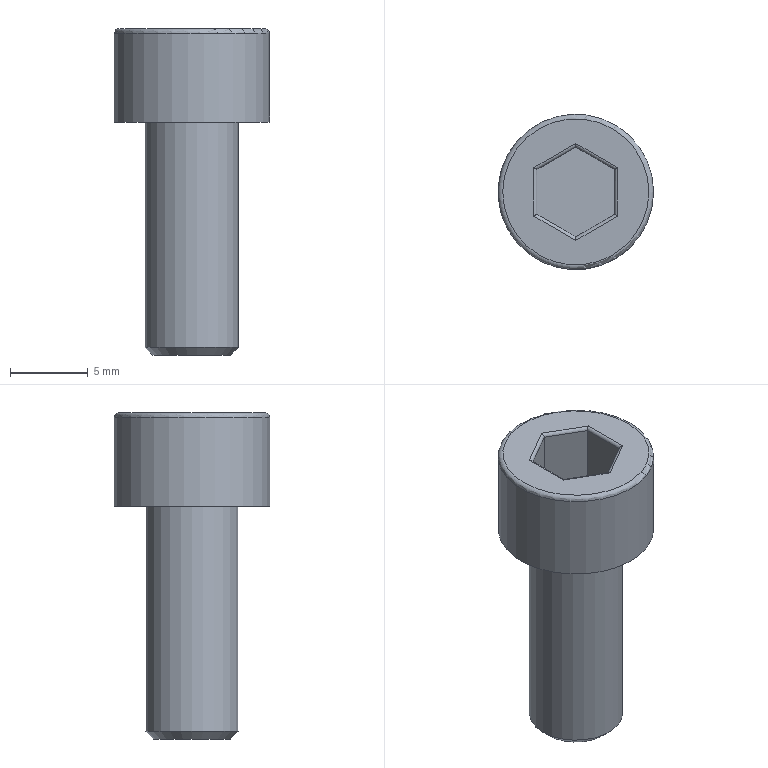Part | STEP file | 200 mesh_id126_x | 1 solid | 20 faces | box 10 x 10 x 21 mm | volume 805.776 mm3 | plane 10 | cylinder 8 | torus 1 | cone 1 | commonest cylinder face diameters 0.4 x6 6 x1 10 x1
STEP:
#1=CARTESIAN_POINT('',(-17007.884,-4107.151,86.258));
#2=VERTEX_POINT('',#1);
#3=CARTESIAN_POINT('',(-17005.184,-4108.71,86.258));
#4=VERTEX_POINT('',#3);
#5=CARTESIAN_POINT('',(-17005.284,-4108.653,86.258));
#6=DIRECTION('',(0.866,-0.5,0.));
#7=VECTOR('',#6,1.);
#8=LINE('',#5,#7);
#9=EDGE_CURVE('',#2,#4,#8,.T.);
#10=ORIENTED_EDGE('',*,*,#9,.T.);
#11=CARTESIAN_POINT('',(-17005.184,-4111.828,86.258));
#12=VERTEX_POINT('',#11);
#13=CARTESIAN_POINT('',(-17005.184,-4111.713,86.258));
#14=DIRECTION('',(0.,-1.,0.));
#15=VECTOR('',#14,1.);
#16=LINE('',#13,#15);
#17=EDGE_CURVE('',#4,#12,#16,.T.);
#18=ORIENTED_EDGE('',*,*,#17,.T.);
#19=CARTESIAN_POINT('',(-17007.884,-4113.387,86.258));
#20=VERTEX_POINT('',#19);
#21=CARTESIAN_POINT('',(-17007.784,-4113.329,86.258));
#22=DIRECTION('',(-0.866,-0.5,0.));
#23=VECTOR('',#22,1.);
#24=LINE('',#21,#23);
#25=EDGE_CURVE('',#12,#20,#24,.T.);
#26=ORIENTED_EDGE('',*,*,#25,.T.);
#27=CARTESIAN_POINT('',(-17010.584,-4111.828,86.258));
#28=VERTEX_POINT('',#27);
#29=CARTESIAN_POINT('',(-17010.484,-4111.886,86.258));
#30=DIRECTION('',(-0.866,0.5,0.));
#31=VECTOR('',#30,1.);
#32=LINE('',#29,#31);
#33=EDGE_CURVE('',#20,#28,#32,.T.);
#34=ORIENTED_EDGE('',*,*,#33,.T.);
#35=CARTESIAN_POINT('',(-17010.584,-4108.71,86.258));
#36=VERTEX_POINT('',#35);
#37=CARTESIAN_POINT('',(-17010.584,-4108.826,86.258));
#38=DIRECTION('',(0.,1.,0.));
#39=VECTOR('',#38,1.);
#40=LINE('',#37,#39);
#41=EDGE_CURVE('',#28,#36,#40,.T.);
#42=ORIENTED_EDGE('',*,*,#41,.T.);
#43=CARTESIAN_POINT('',(-17007.984,-4107.209,86.258));
#44=DIRECTION('',(0.866,0.5,0.));
#45=VECTOR('',#44,1.);
#46=LINE('',#43,#45);
#47=EDGE_CURVE('',#36,#2,#46,.T.);
#48=ORIENTED_EDGE('',*,*,#47,.T.);
#49=EDGE_LOOP('',(#10,#18,#26,#34,#42,#48));
#50=FACE_BOUND('',#49,.T.);
#51=CARTESIAN_POINT('',(-17003.184,-4110.269,86.258));
#52=VERTEX_POINT('',#51);
#53=CARTESIAN_POINT('',(-17007.884,-4110.269,86.258));
#54=DIRECTION('',(0.,0.,1.));
#55=DIRECTION('',(1.,0.,0.));
#56=AXIS2_PLACEMENT_3D('',#53,#54,#55);
#57=CIRCLE('',#56,4.7);
#58=EDGE_CURVE('',#52,#52,#57,.T.);
#59=ORIENTED_EDGE('',*,*,#58,.T.);
#60=EDGE_LOOP('',(#59));
#61=FACE_BOUND('',#60,.T.);
#62=CARTESIAN_POINT('',(-17007.884,-4110.269,86.258));
#63=DIRECTION('',(0.,0.,1.));
#64=DIRECTION('',(1.,0.,0.));
#65=AXIS2_PLACEMENT_3D('',#62,#63,#64);
#66=PLANE('',#65);
#67=ADVANCED_FACE('',(#50,#61),#66,.T.);
#68=CARTESIAN_POINT('',(-17010.884,-4110.269,80.258));
#69=VERTEX_POINT('',#68);
#70=CARTESIAN_POINT('',(-17007.884,-4110.269,80.258));
#71=DIRECTION('',(0.,0.,-1.));
#72=DIRECTION('',(-1.,0.,0.));
#73=AXIS2_PLACEMENT_3D('',#70,#71,#72);
#74=CIRCLE('',#73,3.);
#75=EDGE_CURVE('',#69,#69,#74,.T.);
#76=ORIENTED_EDGE('',*,*,#75,.F.);
#77=EDGE_LOOP('',(#76));
#78=FACE_BOUND('',#77,.T.);
#79=CARTESIAN_POINT('',(-17002.884,-4110.269,80.258));
#80=VERTEX_POINT('',#79);
#81=CARTESIAN_POINT('',(-17007.884,-4110.269,80.258));
#82=DIRECTION('',(0.,0.,1.));
#83=DIRECTION('',(1.,0.,0.));
#84=AXIS2_PLACEMENT_3D('',#81,#82,#83);
#85=CIRCLE('',#84,5.);
#86=EDGE_CURVE('',#80,#80,#85,.T.);
#87=ORIENTED_EDGE('',*,*,#86,.F.);
#88=EDGE_LOOP('',(#87));
#89=FACE_BOUND('',#88,.T.);
#90=CARTESIAN_POINT('',(-17007.884,-4110.269,80.258));
#91=DIRECTION('',(0.,0.,-1.));
#92=DIRECTION('',(-1.,0.,0.));
#93=AXIS2_PLACEMENT_3D('',#90,#91,#92);
#94=PLANE('',#93);
#95=ADVANCED_FACE('',(#78,#89),#94,.T.);
#96=CARTESIAN_POINT('',(-17002.884,-4110.269,85.958));
#97=VERTEX_POINT('',#96);
#98=CARTESIAN_POINT('',(-17007.884,-4110.269,85.958));
#99=DIRECTION('',(0.,0.,-1.));
#100=DIRECTION('',(1.,0.,0.));
#101=AXIS2_PLACEMENT_3D('',#98,#99,#100);
#102=CIRCLE('',#101,5.);
#103=EDGE_CURVE('',#97,#97,#102,.T.);
#104=ORIENTED_EDGE('',*,*,#103,.T.);
#105=EDGE_LOOP('',(#104));
#106=FACE_BOUND('',#105,.T.);
#107=ORIENTED_EDGE('',*,*,#86,.T.);
#108=EDGE_LOOP('',(#107));
#109=FACE_BOUND('',#108,.T.);
#110=CARTESIAN_POINT('',(-17007.884,-4110.269,80.258));
#111=DIRECTION('',(0.,0.,1.));
#112=DIRECTION('',(1.,0.,0.));
#113=AXIS2_PLACEMENT_3D('',#110,#111,#112);
#114=CYLINDRICAL_SURFACE('',#113,5.);
#115=ADVANCED_FACE('',(#106,#109),#114,.T.);
#116=CARTESIAN_POINT('',(-17005.384,-4108.826,86.058));
#117=VERTEX_POINT('',#116);
#118=CARTESIAN_POINT('',(-17005.384,-4108.826,82.258));
#119=VERTEX_POINT('',#118);
#120=CARTESIAN_POINT('',(-17005.384,-4108.826,82.258));
#121=DIRECTION('',(0.,0.,-1.));
#122=VECTOR('',#121,1.);
#123=LINE('',#120,#122);
#124=EDGE_CURVE('',#117,#119,#123,.T.);
#125=ORIENTED_EDGE('',*,*,#124,.F.);
#126=CARTESIAN_POINT('',(-17007.884,-4107.382,86.058));
#127=VERTEX_POINT('',#126);
#128=CARTESIAN_POINT('',(-17007.884,-4107.382,86.058));
#129=DIRECTION('',(-0.866,0.5,0.));
#130=VECTOR('',#129,1.);
#131=LINE('',#128,#130);
#132=EDGE_CURVE('',#117,#127,#131,.T.);
#133=ORIENTED_EDGE('',*,*,#132,.T.);
#134=CARTESIAN_POINT('',(-17007.884,-4107.382,82.258));
#135=VERTEX_POINT('',#134);
#136=CARTESIAN_POINT('',(-17007.884,-4107.382,82.258));
#137=DIRECTION('',(0.,0.,-1.));
#138=VECTOR('',#137,1.);
#139=LINE('',#136,#138);
#140=EDGE_CURVE('',#127,#135,#139,.T.);
#141=ORIENTED_EDGE('',*,*,#140,.T.);
#142=CARTESIAN_POINT('',(-17005.384,-4108.826,82.258));
#143=DIRECTION('',(0.866,-0.5,0.));
#144=VECTOR('',#143,1.);
#145=LINE('',#142,#144);
#146=EDGE_CURVE('',#135,#119,#145,.T.);
#147=ORIENTED_EDGE('',*,*,#146,.T.);
#148=EDGE_LOOP('',(#125,#133,#141,#147));
#149=FACE_OUTER_BOUND('',#148,.T.);
#150=CARTESIAN_POINT('',(-17005.384,-4108.826,82.258));
#151=DIRECTION('',(0.5,0.866,0.));
#152=DIRECTION('',(-0.866,0.5,0.));
#153=AXIS2_PLACEMENT_3D('',#150,#151,#152);
#154=PLANE('',#153);
#155=ADVANCED_FACE('',(#149),#154,.F.);
#156=ORIENTED_EDGE('',*,*,#140,.F.);
#157=CARTESIAN_POINT('',(-17010.384,-4108.826,86.058));
#158=VERTEX_POINT('',#157);
#159=CARTESIAN_POINT('',(-17010.384,-4108.826,86.058));
#160=DIRECTION('',(-0.866,-0.5,0.));
#161=VECTOR('',#160,1.);
#162=LINE('',#159,#161);
#163=EDGE_CURVE('',#127,#158,#162,.T.);
#164=ORIENTED_EDGE('',*,*,#163,.T.);
#165=CARTESIAN_POINT('',(-17010.384,-4108.826,82.258));
#166=VERTEX_POINT('',#165);
#167=CARTESIAN_POINT('',(-17010.384,-4108.826,82.258));
#168=DIRECTION('',(0.,0.,-1.));
#169=VECTOR('',#168,1.);
#170=LINE('',#167,#169);
#171=EDGE_CURVE('',#158,#166,#170,.T.);
#172=ORIENTED_EDGE('',*,*,#171,.T.);
#173=CARTESIAN_POINT('',(-17007.884,-4107.382,82.258));
#174=DIRECTION('',(0.866,0.5,0.));
#175=VECTOR('',#174,1.);
#176=LINE('',#173,#175);
#177=EDGE_CURVE('',#166,#135,#176,.T.);
#178=ORIENTED_EDGE('',*,*,#177,.T.);
#179=EDGE_LOOP('',(#156,#164,#172,#178));
#180=FACE_OUTER_BOUND('',#179,.T.);
#181=CARTESIAN_POINT('',(-17007.884,-4107.382,82.258));
#182=DIRECTION('',(-0.5,0.866,0.));
#183=DIRECTION('',(-0.866,-0.5,0.));
#184=AXIS2_PLACEMENT_3D('',#181,#182,#183);
#185=PLANE('',#184);
#186=ADVANCED_FACE('',(#180),#185,.F.);
#187=ORIENTED_EDGE('',*,*,#171,.F.);
#188=CARTESIAN_POINT('',(-17010.384,-4111.713,86.058));
#189=VERTEX_POINT('',#188);
#190=CARTESIAN_POINT('',(-17010.384,-4111.713,86.058));
#191=DIRECTION('',(0.,-1.,0.));
#192=VECTOR('',#191,1.);
#193=LINE('',#190,#192);
#194=EDGE_CURVE('',#158,#189,#193,.T.);
#195=ORIENTED_EDGE('',*,*,#194,.T.);
#196=CARTESIAN_POINT('',(-17010.384,-4111.713,82.258));
#197=VERTEX_POINT('',#196);
#198=CARTESIAN_POINT('',(-17010.384,-4111.713,82.258));
#199=DIRECTION('',(0.,0.,-1.));
#200=VECTOR('',#199,1.);
#201=LINE('',#198,#200);
#202=EDGE_CURVE('',#189,#197,#201,.T.);
#203=ORIENTED_EDGE('',*,*,#202,.T.);
#204=CARTESIAN_POINT('',(-17010.384,-4108.826,82.258));
#205=DIRECTION('',(0.,1.,0.));
#206=VECTOR('',#205,1.);
#207=LINE('',#204,#206);
#208=EDGE_CURVE('',#197,#166,#207,.T.);
#209=ORIENTED_EDGE('',*,*,#208,.T.);
#210=EDGE_LOOP('',(#187,#195,#203,#209));
#211=FACE_OUTER_BOUND('',#210,.T.);
#212=CARTESIAN_POINT('',(-17010.384,-4108.826,82.258));
#213=DIRECTION('',(-1.,0.,0.));
#214=DIRECTION('',(0.,0.,1.));
#215=AXIS2_PLACEMENT_3D('',#212,#213,#214);
#216=PLANE('',#215);
#217=ADVANCED_FACE('',(#211),#216,.F.);
#218=ORIENTED_EDGE('',*,*,#202,.F.);
#219=CARTESIAN_POINT('',(-17007.884,-4113.156,86.058));
#220=VERTEX_POINT('',#219);
#221=CARTESIAN_POINT('',(-17007.884,-4113.156,86.058));
#222=DIRECTION('',(0.866,-0.5,0.));
#223=VECTOR('',#222,1.);
#224=LINE('',#221,#223);
#225=EDGE_CURVE('',#189,#220,#224,.T.);
#226=ORIENTED_EDGE('',*,*,#225,.T.);
#227=CARTESIAN_POINT('',(-17007.884,-4113.156,82.258));
#228=VERTEX_POINT('',#227);
#229=CARTESIAN_POINT('',(-17007.884,-4113.156,82.258));
#230=DIRECTION('',(0.,0.,-1.));
#231=VECTOR('',#230,1.);
#232=LINE('',#229,#231);
#233=EDGE_CURVE('',#220,#228,#232,.T.);
#234=ORIENTED_EDGE('',*,*,#233,.T.);
#235=CARTESIAN_POINT('',(-17010.384,-4111.713,82.258));
#236=DIRECTION('',(-0.866,0.5,0.));
#237=VECTOR('',#236,1.);
#238=LINE('',#235,#237);
#239=EDGE_CURVE('',#228,#197,#238,.T.);
#240=ORIENTED_EDGE('',*,*,#239,.T.);
#241=EDGE_LOOP('',(#218,#226,#234,#240));
#242=FACE_OUTER_BOUND('',#241,.T.);
#243=CARTESIAN_POINT('',(-17010.384,-4111.713,82.258));
#244=DIRECTION('',(-0.5,-0.866,0.));
#245=DIRECTION('',(0.866,-0.5,0.));
#246=AXIS2_PLACEMENT_3D('',#243,#244,#245);
#247=PLANE('',#246);
#248=ADVANCED_FACE('',(#242),#247,.F.);
#249=ORIENTED_EDGE('',*,*,#233,.F.);
#250=CARTESIAN_POINT('',(-17005.384,-4111.713,86.058));
#251=VERTEX_POINT('',#250);
#252=CARTESIAN_POINT('',(-17005.384,-4111.713,86.058));
#253=DIRECTION('',(0.866,0.5,0.));
#254=VECTOR('',#253,1.);
#255=LINE('',#252,#254);
#256=EDGE_CURVE('',#220,#251,#255,.T.);
#257=ORIENTED_EDGE('',*,*,#256,.T.);
#258=CARTESIAN_POINT('',(-17005.384,-4111.713,82.258));
#259=VERTEX_POINT('',#258);
#260=CARTESIAN_POINT('',(-17005.384,-4111.713,82.258));
#261=DIRECTION('',(0.,0.,-1.));
#262=VECTOR('',#261,1.);
#263=LINE('',#260,#262);
#264=EDGE_CURVE('',#251,#259,#263,.T.);
#265=ORIENTED_EDGE('',*,*,#264,.T.);
#266=CARTESIAN_POINT('',(-17007.884,-4113.156,82.258));
#267=DIRECTION('',(-0.866,-0.5,0.));
#268=VECTOR('',#267,1.);
#269=LINE('',#266,#268);
#270=EDGE_CURVE('',#259,#228,#269,.T.);
#271=ORIENTED_EDGE('',*,*,#270,.T.);
#272=EDGE_LOOP('',(#249,#257,#265,#271));
#273=FACE_OUTER_BOUND('',#272,.T.);
#274=CARTESIAN_POINT('',(-17007.884,-4113.156,82.258));
#275=DIRECTION('',(0.5,-0.866,0.));
#276=DIRECTION('',(0.866,0.5,0.));
#277=AXIS2_PLACEMENT_3D('',#274,#275,#276);
#278=PLANE('',#277);
#279=ADVANCED_FACE('',(#273),#278,.F.);
#280=ORIENTED_EDGE('',*,*,#264,.F.);
#281=CARTESIAN_POINT('',(-17005.384,-4108.826,86.058));
#282=DIRECTION('',(0.,1.,0.));
#283=VECTOR('',#282,1.);
#284=LINE('',#281,#283);
#285=EDGE_CURVE('',#251,#117,#284,.T.);
#286=ORIENTED_EDGE('',*,*,#285,.T.);
#287=ORIENTED_EDGE('',*,*,#124,.T.);
#288=CARTESIAN_POINT('',(-17005.384,-4111.713,82.258));
#289=DIRECTION('',(0.,-1.,0.));
#290=VECTOR('',#289,1.);
#291=LINE('',#288,#290);
#292=EDGE_CURVE('',#119,#259,#291,.T.);
#293=ORIENTED_EDGE('',*,*,#292,.T.);
#294=EDGE_LOOP('',(#280,#286,#287,#293));
#295=FACE_OUTER_BOUND('',#294,.T.);
#296=CARTESIAN_POINT('',(-17005.384,-4111.713,82.258));
#297=DIRECTION('',(1.,0.,0.));
#298=DIRECTION('',(0.,0.,-1.));
#299=AXIS2_PLACEMENT_3D('',#296,#297,#298);
#300=PLANE('',#299);
#301=ADVANCED_FACE('',(#295),#300,.F.);
#302=ORIENTED_EDGE('',*,*,#146,.F.);
#303=ORIENTED_EDGE('',*,*,#177,.F.);
#304=ORIENTED_EDGE('',*,*,#208,.F.);
#305=ORIENTED_EDGE('',*,*,#239,.F.);
#306=ORIENTED_EDGE('',*,*,#270,.F.);
#307=ORIENTED_EDGE('',*,*,#292,.F.);
#308=EDGE_LOOP('',(#302,#303,#304,#305,#306,#307));
#309=FACE_OUTER_BOUND('',#308,.T.);
#310=CARTESIAN_POINT('',(0.,-175.,82.258));
#311=DIRECTION('',(0.,0.,1.));
#312=DIRECTION('',(1.,0.,0.));
#313=AXIS2_PLACEMENT_3D('',#310,#311,#312);
#314=PLANE('',#313);
#315=ADVANCED_FACE('',(#309),#314,.T.);
#316=ORIENTED_EDGE('',*,*,#58,.F.);
#317=EDGE_LOOP('',(#316));
#318=FACE_BOUND('',#317,.T.);
#319=ORIENTED_EDGE('',*,*,#103,.F.);
#320=EDGE_LOOP('',(#319));
#321=FACE_BOUND('',#320,.T.);
#322=CARTESIAN_POINT('',(-17007.884,-4110.269,85.958));
#323=DIRECTION('',(0.,0.,1.));
#324=DIRECTION('',(1.,0.,0.));
#325=AXIS2_PLACEMENT_3D('',#322,#323,#324);
#326=TOROIDAL_SURFACE('',#325,4.7,0.3);
#327=ADVANCED_FACE('',(#318,#321),#326,.T.);
#328=CARTESIAN_POINT('',(-17010.584,-4108.71,86.058));
#329=DIRECTION('',(0.5,0.866,0.));
#330=DIRECTION('',(-0.866,0.5,0.));
#331=AXIS2_PLACEMENT_3D('',#328,#329,#330);
#332=ELLIPSE('',#331,0.2309,0.2);
#333=EDGE_CURVE('',#36,#158,#332,.T.);
#334=ORIENTED_EDGE('',*,*,#333,.F.);
#335=ORIENTED_EDGE('',*,*,#41,.F.);
#336=CARTESIAN_POINT('',(-17010.584,-4111.828,86.058));
#337=DIRECTION('',(0.5,-0.866,0.));
#338=DIRECTION('',(-0.866,-0.5,0.));
#339=AXIS2_PLACEMENT_3D('',#336,#337,#338);
#340=ELLIPSE('',#339,0.2309,0.2);
#341=EDGE_CURVE('',#189,#28,#340,.T.);
#342=ORIENTED_EDGE('',*,*,#341,.F.);
#343=ORIENTED_EDGE('',*,*,#194,.F.);
#344=EDGE_LOOP('',(#334,#335,#342,#343));
#345=FACE_OUTER_BOUND('',#344,.T.);
#346=CARTESIAN_POINT('',(-17010.584,-4108.826,86.058));
#347=DIRECTION('',(0.,1.,0.));
#348=DIRECTION('',(0.,0.,1.));
#349=AXIS2_PLACEMENT_3D('',#346,#347,#348);
#350=CYLINDRICAL_SURFACE('',#349,0.2);
#351=ADVANCED_FACE('',(#345),#350,.T.);
#352=ORIENTED_EDGE('',*,*,#341,.T.);
#353=ORIENTED_EDGE('',*,*,#33,.F.);
#354=CARTESIAN_POINT('',(-17007.884,-4113.387,86.058));
#355=DIRECTION('',(1.,0.,0.));
#356=DIRECTION('',(0.,-1.,0.));
#357=AXIS2_PLACEMENT_3D('',#354,#355,#356);
#358=ELLIPSE('',#357,0.2309,0.2);
#359=EDGE_CURVE('',#220,#20,#358,.T.);
#360=ORIENTED_EDGE('',*,*,#359,.F.);
#361=ORIENTED_EDGE('',*,*,#225,.F.);
#362=EDGE_LOOP('',(#352,#353,#360,#361));
#363=FACE_OUTER_BOUND('',#362,.T.);
#364=CARTESIAN_POINT('',(-17010.484,-4111.886,86.058));
#365=DIRECTION('',(-0.866,0.5,0.));
#366=DIRECTION('',(-0.5,-0.866,0.));
#367=AXIS2_PLACEMENT_3D('',#364,#365,#366);
#368=CYLINDRICAL_SURFACE('',#367,0.2);
#369=ADVANCED_FACE('',(#363),#368,.T.);
#370=ORIENTED_EDGE('',*,*,#333,.T.);
#371=ORIENTED_EDGE('',*,*,#163,.F.);
#372=CARTESIAN_POINT('',(-17007.884,-4107.151,86.058));
#373=DIRECTION('',(1.,0.,0.));
#374=DIRECTION('',(0.,1.,0.));
#375=AXIS2_PLACEMENT_3D('',#372,#373,#374);
#376=ELLIPSE('',#375,0.2309,0.2);
#377=EDGE_CURVE('',#2,#127,#376,.T.);
#378=ORIENTED_EDGE('',*,*,#377,.F.);
#379=ORIENTED_EDGE('',*,*,#47,.F.);
#380=EDGE_LOOP('',(#370,#371,#378,#379));
#381=FACE_OUTER_BOUND('',#380,.T.);
#382=CARTESIAN_POINT('',(-17007.984,-4107.209,86.058));
#383=DIRECTION('',(0.866,0.5,0.));
#384=DIRECTION('',(-0.5,0.866,0.));
#385=AXIS2_PLACEMENT_3D('',#382,#383,#384);
#386=CYLINDRICAL_SURFACE('',#385,0.2);
#387=ADVANCED_FACE('',(#381),#386,.T.);
#388=ORIENTED_EDGE('',*,*,#359,.T.);
#389=ORIENTED_EDGE('',*,*,#25,.F.);
#390=CARTESIAN_POINT('',(-17005.184,-4111.828,86.058));
#391=DIRECTION('',(0.5,0.866,0.));
#392=DIRECTION('',(0.866,-0.5,0.));
#393=AXIS2_PLACEMENT_3D('',#390,#391,#392);
#394=ELLIPSE('',#393,0.2309,0.2);
#395=EDGE_CURVE('',#251,#12,#394,.T.);
#396=ORIENTED_EDGE('',*,*,#395,.F.);
#397=ORIENTED_EDGE('',*,*,#256,.F.);
#398=EDGE_LOOP('',(#388,#389,#396,#397));
#399=FACE_OUTER_BOUND('',#398,.T.);
#400=CARTESIAN_POINT('',(-17007.784,-4113.329,86.058));
#401=DIRECTION('',(-0.866,-0.5,0.));
#402=DIRECTION('',(0.5,-0.866,0.));
#403=AXIS2_PLACEMENT_3D('',#400,#401,#402);
#404=CYLINDRICAL_SURFACE('',#403,0.2);
#405=ADVANCED_FACE('',(#399),#404,.T.);
#406=ORIENTED_EDGE('',*,*,#377,.T.);
#407=ORIENTED_EDGE('',*,*,#132,.F.);
#408=CARTESIAN_POINT('',(-17005.184,-4108.71,86.058));
#409=DIRECTION('',(0.5,-0.866,0.));
#410=DIRECTION('',(-0.866,-0.5,0.));
#411=AXIS2_PLACEMENT_3D('',#408,#409,#410);
#412=ELLIPSE('',#411,0.2309,0.2);
#413=EDGE_CURVE('',#4,#117,#412,.T.);
#414=ORIENTED_EDGE('',*,*,#413,.F.);
#415=ORIENTED_EDGE('',*,*,#9,.F.);
#416=EDGE_LOOP('',(#406,#407,#414,#415));
#417=FACE_OUTER_BOUND('',#416,.T.);
#418=CARTESIAN_POINT('',(-17005.284,-4108.653,86.058));
#419=DIRECTION('',(0.866,-0.5,0.));
#420=DIRECTION('',(0.5,0.866,0.));
#421=AXIS2_PLACEMENT_3D('',#418,#419,#420);
#422=CYLINDRICAL_SURFACE('',#421,0.2);
#423=ADVANCED_FACE('',(#417),#422,.T.);
#424=ORIENTED_EDGE('',*,*,#395,.T.);
#425=ORIENTED_EDGE('',*,*,#17,.F.);
#426=ORIENTED_EDGE('',*,*,#413,.T.);
#427=ORIENTED_EDGE('',*,*,#285,.F.);
#428=EDGE_LOOP('',(#424,#425,#426,#427));
#429=FACE_OUTER_BOUND('',#428,.T.);
#430=CARTESIAN_POINT('',(-17005.184,-4111.713,86.058));
#431=DIRECTION('',(0.,-1.,0.));
#432=DIRECTION('',(0.,0.,-1.));
#433=AXIS2_PLACEMENT_3D('',#430,#431,#432);
#434=CYLINDRICAL_SURFACE('',#433,0.2);
#435=ADVANCED_FACE('',(#429),#434,.T.);
#436=CARTESIAN_POINT('',(-17010.884,-4110.269,65.758));
#437=VERTEX_POINT('',#436);
#438=CARTESIAN_POINT('',(-17007.884,-4110.269,65.758));
#439=DIRECTION('',(0.,0.,1.));
#440=DIRECTION('',(-1.,0.,0.));
#441=AXIS2_PLACEMENT_3D('',#438,#439,#440);
#442=CIRCLE('',#441,3.);
#443=EDGE_CURVE('',#437,#437,#442,.T.);
#444=ORIENTED_EDGE('',*,*,#443,.T.);
#445=EDGE_LOOP('',(#444));
#446=FACE_BOUND('',#445,.T.);
#447=ORIENTED_EDGE('',*,*,#75,.T.);
#448=EDGE_LOOP('',(#447));
#449=FACE_BOUND('',#448,.T.);
#450=CARTESIAN_POINT('',(-17007.884,-4110.269,65.258));
#451=DIRECTION('',(0.,0.,1.));
#452=DIRECTION('',(1.,0.,0.));
#453=AXIS2_PLACEMENT_3D('',#450,#451,#452);
#454=CYLINDRICAL_SURFACE('',#453,3.);
#455=ADVANCED_FACE('',(#446,#449),#454,.T.);
#456=CARTESIAN_POINT('',(-17010.384,-4110.269,65.258));
#457=VERTEX_POINT('',#456);
#458=CARTESIAN_POINT('',(-17007.884,-4110.269,65.258));
#459=DIRECTION('',(0.,0.,-1.));
#460=DIRECTION('',(-1.,0.,0.));
#461=AXIS2_PLACEMENT_3D('',#458,#459,#460);
#462=CIRCLE('',#461,2.5);
#463=EDGE_CURVE('',#457,#457,#462,.T.);
#464=ORIENTED_EDGE('',*,*,#463,.T.);
#465=EDGE_LOOP('',(#464));
#466=FACE_OUTER_BOUND('',#465,.T.);
#467=CARTESIAN_POINT('',(-17007.884,-4110.269,65.258));
#468=DIRECTION('',(0.,0.,-1.));
#469=DIRECTION('',(-1.,0.,0.));
#470=AXIS2_PLACEMENT_3D('',#467,#468,#469);
#471=PLANE('',#470);
#472=ADVANCED_FACE('',(#466),#471,.T.);
#473=ORIENTED_EDGE('',*,*,#443,.F.);
#474=EDGE_LOOP('',(#473));
#475=FACE_BOUND('',#474,.T.);
#476=ORIENTED_EDGE('',*,*,#463,.F.);
#477=EDGE_LOOP('',(#476));
#478=FACE_BOUND('',#477,.T.);
#479=CARTESIAN_POINT('',(-17007.884,-4110.269,65.258));
#480=DIRECTION('',(0.,0.,1.));
#481=DIRECTION('',(1.,0.,0.));
#482=AXIS2_PLACEMENT_3D('',#479,#480,#481);
#483=CONICAL_SURFACE('',#482,2.5,45.);
#484=ADVANCED_FACE('',(#475,#478),#483,.T.);
#485=CLOSED_SHELL('',(#67,#95,#115,#155,#186,#217,#248,#279,#301,#315,#327,#351,#369,#387,#405,#423,#435,#455,#472,#484));
#486=MANIFOLD_SOLID_BREP('',#485);
#487=(LENGTH_UNIT()NAMED_UNIT(*)SI_UNIT(.MILLI.,.METRE.));
#488=UNCERTAINTY_MEASURE_WITH_UNIT(LENGTH_MEASURE(0.00002),#487,'','');
#489=(NAMED_UNIT(*)PLANE_ANGLE_UNIT()SI_UNIT($,.RADIAN.));
#490=PLANE_ANGLE_MEASURE_WITH_UNIT(PLANE_ANGLE_MEASURE(0.01745),#489);
#491=DIMENSIONAL_EXPONENTS(0.,0.,0.,0.,0.,0.,0.);
#492=(CONVERSION_BASED_UNIT('DEGREE',#490)NAMED_UNIT(#491)PLANE_ANGLE_UNIT());
#493=(NAMED_UNIT(*)SI_UNIT($,.STERADIAN.)SOLID_ANGLE_UNIT());
#494=(GEOMETRIC_REPRESENTATION_CONTEXT(3)GLOBAL_UNCERTAINTY_ASSIGNED_CONTEXT((#488))GLOBAL_UNIT_ASSIGNED_CONTEXT((#487,#492,#493))REPRESENTATION_CONTEXT('',''));
#495=ADVANCED_BREP_SHAPE_REPRESENTATION('',(#486),#494);